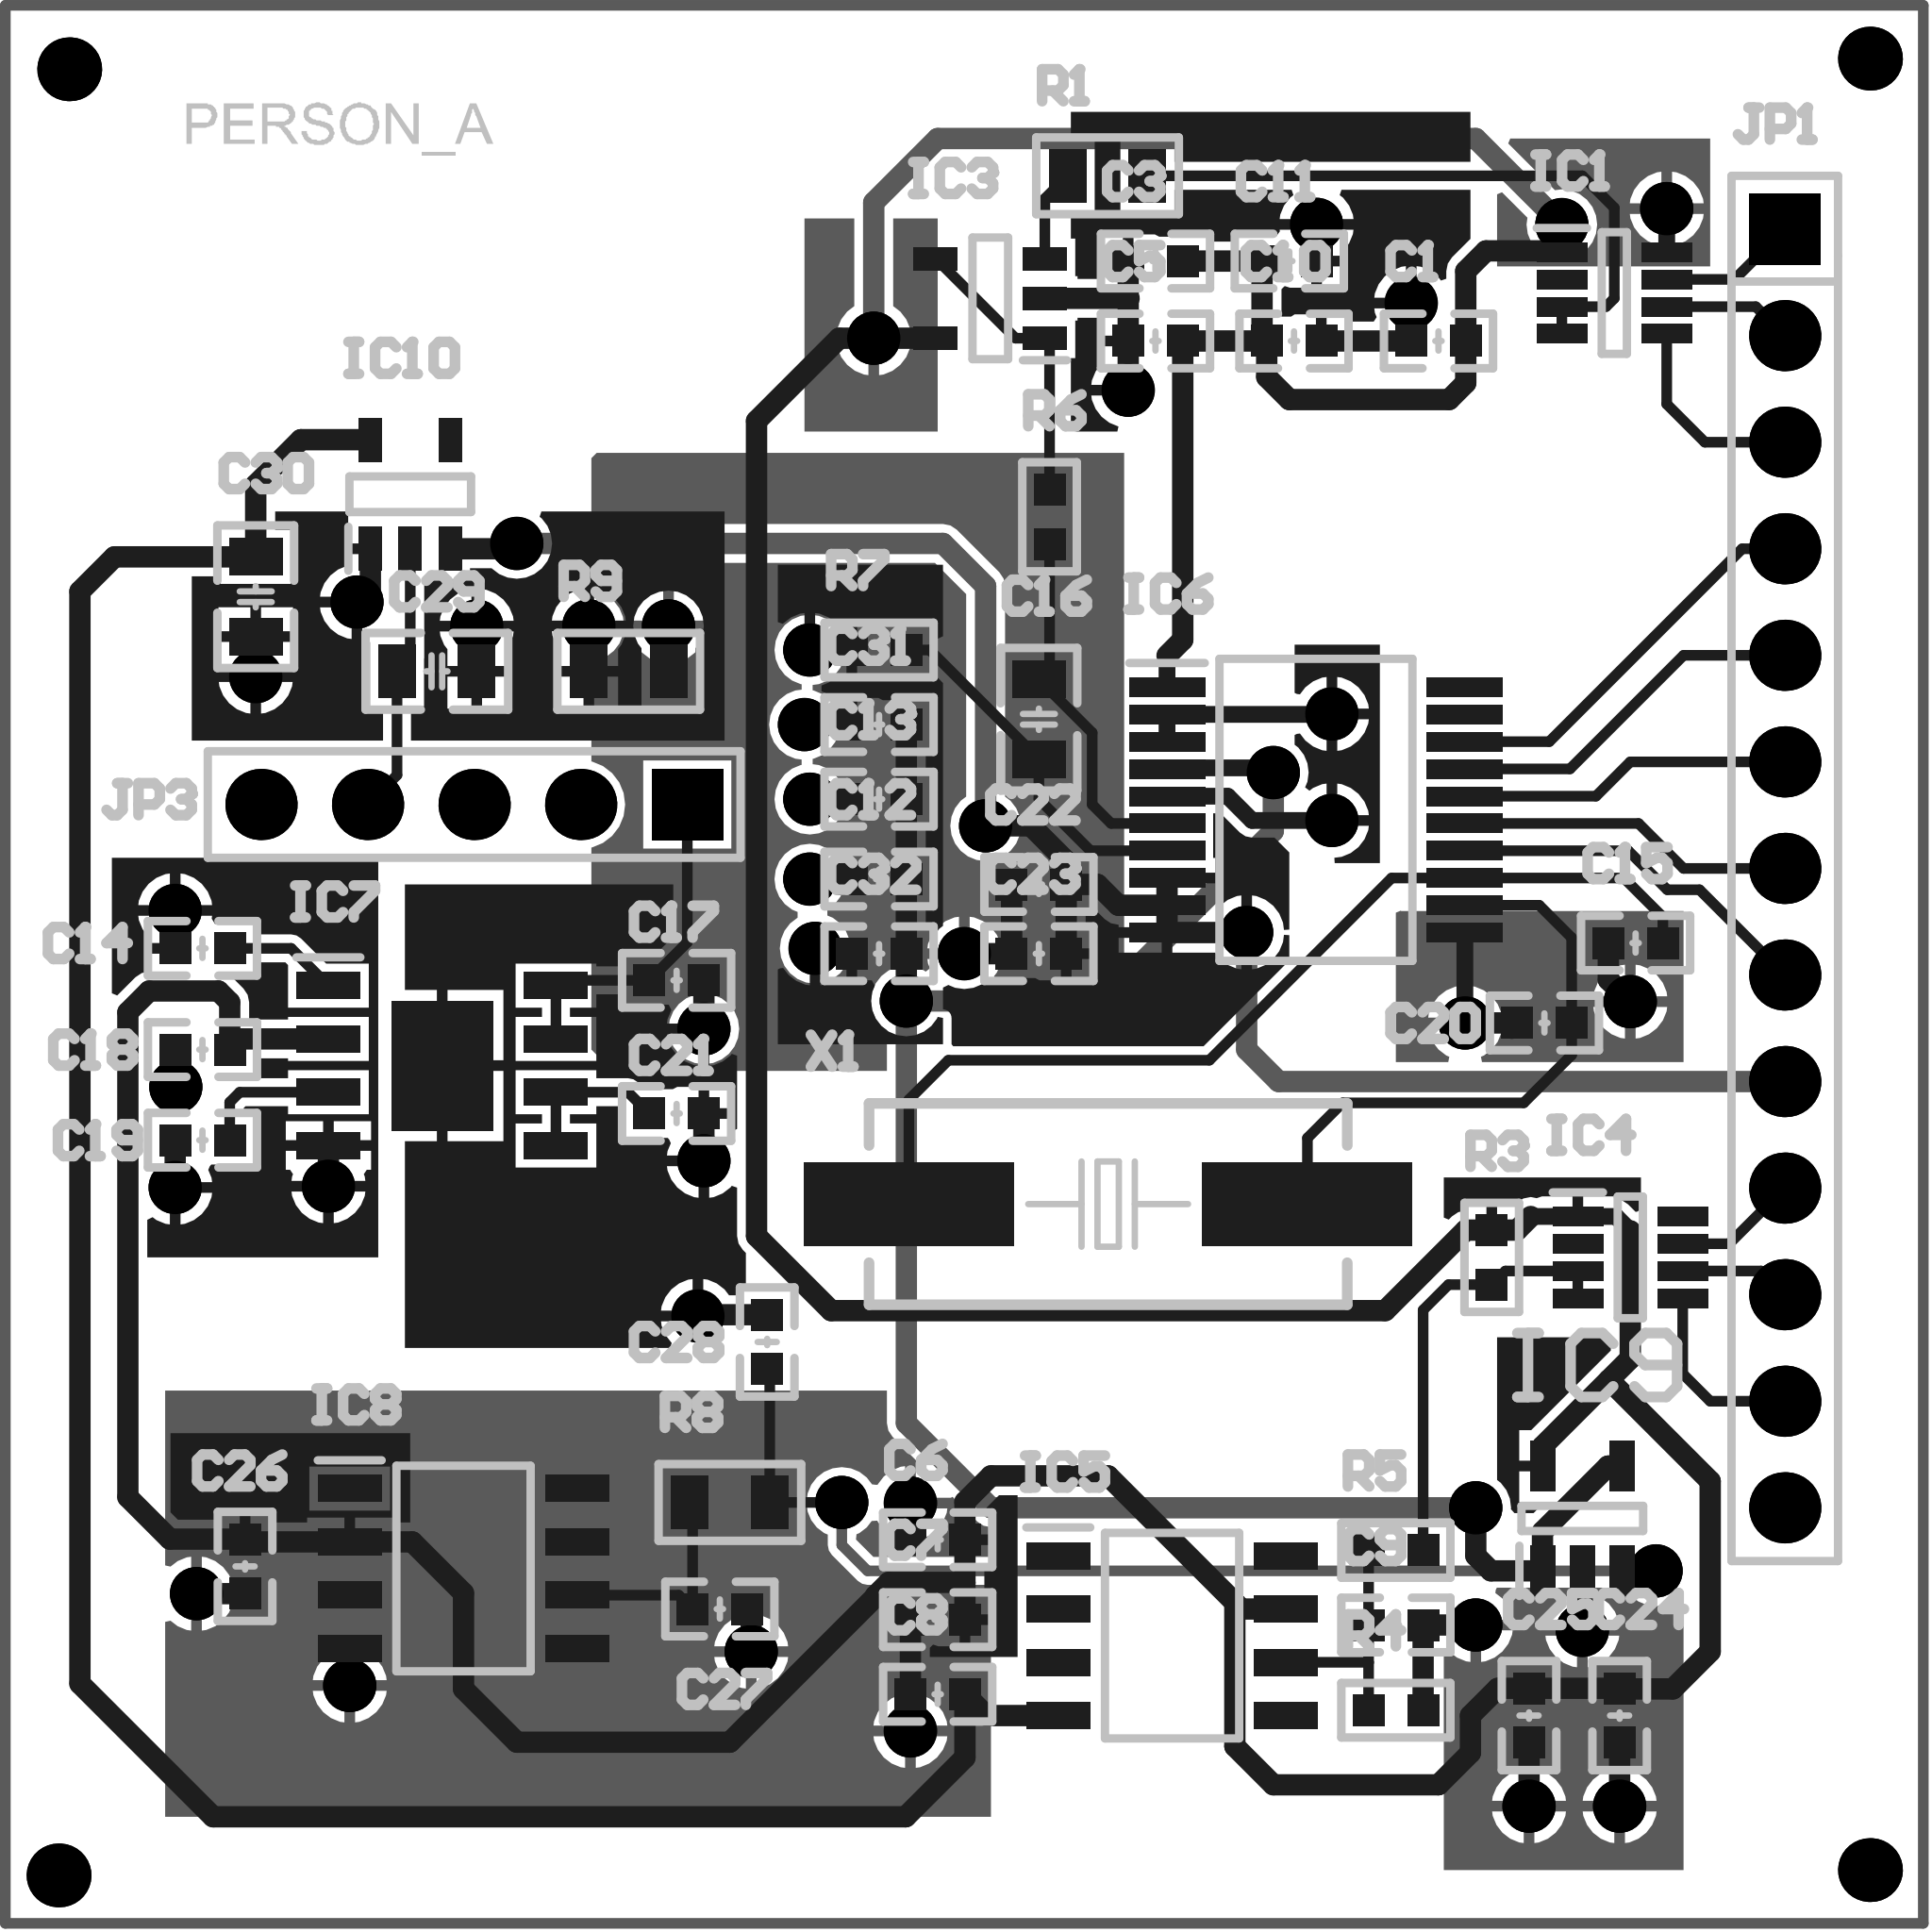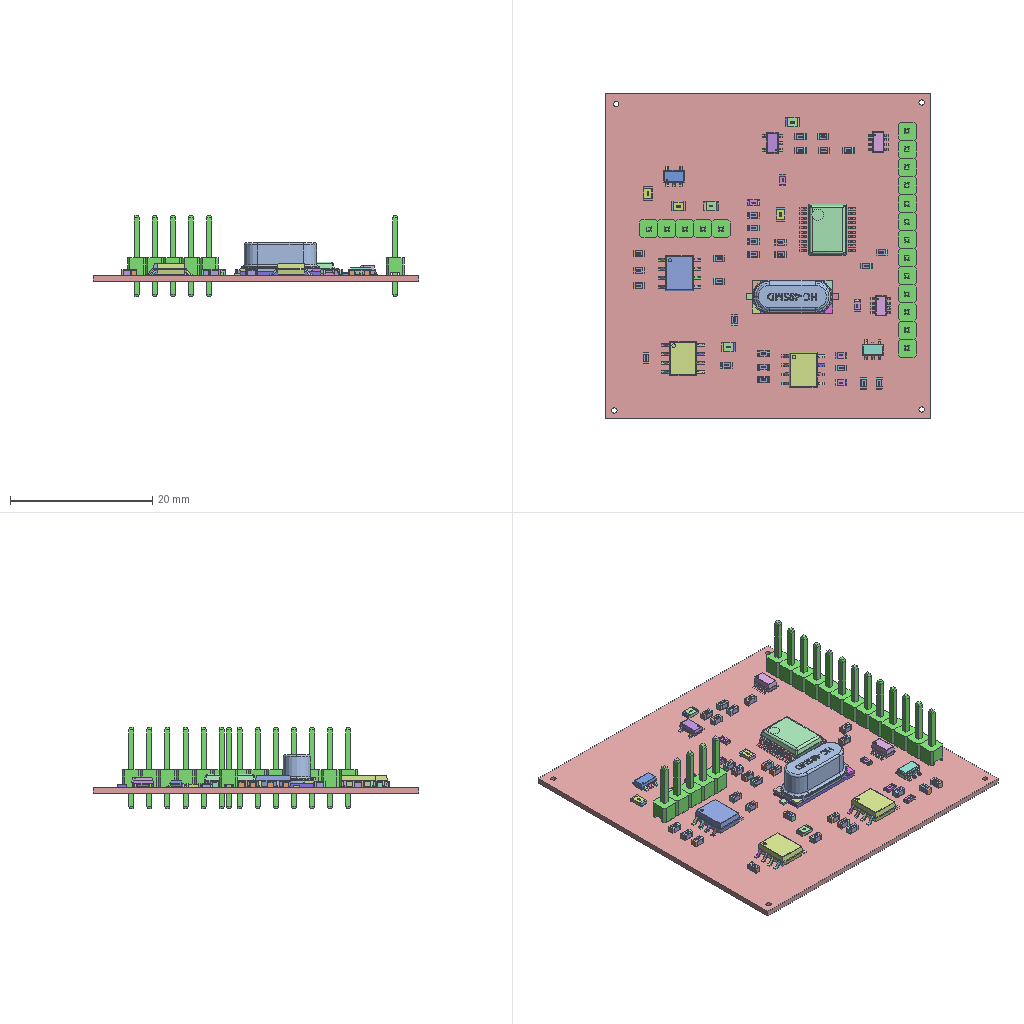Circuit board layout | Altium Designer | box 45.7 x 45.7 x 11.5 mm
Layer stack:
# Altium Designer layer stack of  (unit mm; dielectric type: 0 none, 1 core, 2 prepreg, 3 surface material)
index,name,kind,layer,copper_thickness_mm,dielectric_type,dielectric_thickness_mm,dielectric_material,dielectric_constant
0,Top Paste,other,,,,,,
1,Top Overlay,other,,,,,,
2,Top Solder,dielectric,,,3,0.0102,Solder Resist,3.5
3,Top Layer,copper,Top Layer,0.0356,,,,
4,Dielectric 1,dielectric,,,1,0.254,FR-4,4.2
5,GND,copper,GND,0.036,,,,
6,Dielectric 3,dielectric,,,2,0.127,,4.2
7,PWR,copper,PWR,0.036,,,,
8,Dielectric 2,dielectric,,,1,0.254,,4.2
9,Bottom Layer,copper,Bottom Layer,0.0356,,,,
10,Bottom Solder,dielectric,,,3,0.0102,Solder Resist,3.5
11,Bottom Overlay,other,,,,,,
12,Bottom Paste,other,,,,,,
# drill layer pairs: low layer,high layer
drill_pair,Top Layer,Bottom Layer
Part placement:
Designator,Comment,Layer,Footprint,Center-X(mm),Center-Y(mm),Rotation
IC7,ADM7150ARDZ-5.0-R7,TopLayer,SOIC127P600X175-9N,10.414,20.447,360
C1,0.1uF,TopLayer,C_0603_L,34.163,37.719,180
C6,0.1uF,TopLayer,C_0603_L,22.225,9.144,180
C7,0.1uF,TopLayer,C_0603_L,22.225,7.239,180
C8,0.1uF,TopLayer,C_0603_L,22.225,5.461,360
C9,0.1uF,TopLayer,C_0603_L,33.147,7.112,360
C12,1uF,TopLayer,C_0603_L,20.828,24.892,180
C13,100nF,TopLayer,C_0603_L,20.828,26.797,180
C14,10uF,TopLayer,C_0603_L,4.699,23.241,180
C15,20pF,TopLayer,C_0603_L,38.862,23.368,180
C16,220pF,TopLayer,C_0805_L,24.638,28.702,90
C17,10uF,TopLayer,C_0603_L,16.002,22.479,360
C18,10uF,TopLayer,C_0603_L,4.699,20.828,180
C19,1uF,TopLayer,C_0603_L,4.699,18.669,180
C20,20pF,TopLayer,C_0603_L,36.688,21.463,180
C21,1uF,TopLayer,C_0603_L,16.002,19.304,360
C22,100nF,TopLayer,C_0603_L,24.638,24.765,180
C23,1uF,TopLayer,C_0603_L,24.638,23.114,180
C24,1uF,TopLayer,C_0603_L,38.481,4.953,270
C25,100nF,TopLayer,C_0603_L,36.322,4.953,270
C26,100nF,TopLayer,C_0603_L,5.715,8.509,270
C27,100nF,TopLayer,C_0603_L,17.033,7.493,360
C28,100nF,TopLayer,C_0603_L,18.161,13.858,90
C29,2.2uF,TopLayer,C_0805_L,10.287,29.845,180
C30,2.2uF,TopLayer,C_0805_L,5.969,31.623,270
C31,10uF,TopLayer,C_0603_L,20.828,28.575,360
C32,100nF,TopLayer,C_0603_L,20.828,23.114,360
IC1,AD5660ARJZ-2500RL7,TopLayer,SOT65P280X145-8N,38.354,38.862,360
IC4,AD5660ARJZ-2500RL7,TopLayer,SOT65P280X145-8N,38.735,15.875,0
IC6,ADS1255IDBR,TopLayer,SOP65P780X200-20N,31.242,26.543,0
IC10,ADP7182AUJZ-5.0-R7,TopLayer,SOT95P280X100-5N,9.652,34.066,90
JP1,HDR-1X13,TopLayer,HDR2.54-LI-13P,42.418,25.146,270
JP3,HDR-1X5,TopLayer,HDR2.54-LI-5P,11.176,26.67,180
R3,10K,TopLayer,R_0603_L,35.433,15.875,90
R4,1K,TopLayer,R_0603_L,33.147,5.08,180
R5,10K,TopLayer,R_0603_L,33.147,8.89,360
R6,10R,TopLayer,R_0603_L,24.892,33.528,270
R7,10R,TopLayer,R_0603_L,20.828,30.353,0
R8,10K,TopLayer,R_0805_L,17.272,10.033,360
R9,0R,TopLayer,R_0805_L,14.859,29.845,360
X1,7.68MHz,TopLayer,OSC_HC-49SMD,26.289,17.145,180
IC8,ADR4525ARZ,TopLayer,SOIC127P600X175-8N,10.922,8.458,0
IC5,AD820ARZ,TopLayer,SOIC127P600X175-8N,27.813,6.858,360
C3,100nF,TopLayer,C_0603_L,27.417,39.624,180
C5,1uF,TopLayer,C_0603_L,27.417,37.719,180
C10,1uF,TopLayer,C_0603_L,30.719,37.719,360
C11,100nF,TopLayer,C_0603_L,30.607,39.624,360
IC3,OPA387DBVT,TopLayer,SOT95P280X100-5N,23.48,38.735,180
R1,50R,TopLayer,R_0805_L,26.274,41.656,180
IC9,OPA387DBVT,TopLayer,SOT95P280X145-5N,37.592,9.652,90
Pad and via stacks:
# Altium Designer via and pad stacks of  (unit mm). Each distinct definition once, with the count of objects using it.
# via: kind,start_layer,end_layer,hole_mm,diameter_mm,mode(0 simple;1 top-mid-bottom;2 full stack),diameter_per_layer,count,example_net
# pad: kind,layer,hole_mm,hole_type(0 round;1 square;2 slot),plating,top_size,top_shape(1 round;2 rect;3 octagon;9 rounded rect),mid_size,bottom_size,mode,footprint,size_per_layer,count,example
pad,Top Layer,0,0,plated,0.762x0.762,2,0.762x0.762,0.762x0.762,0,C 0603_L,,54,C32.1
pad,Top Layer,0,0,plated,1.27x0.889,2,1.27x0.889,1.27x0.889,0,C 0805_L,,6,C29.1
pad,Top Layer,0,0,unplated,1.525x0.65,2,1.525x0.65,1.525x0.65,0,SOIC127P600X175-9N,,8,IC7.1
pad,Top Layer,0,0,unplated,3.098x2.41,2,3.098x2.41,3.098x2.41,0,SOIC127P600X175-9N,,1,IC7.9
pad,Top Layer,0,0,unplated,1.525x0.65,2,1.525x0.65,1.525x0.65,0,SOIC127P600X175-8N,,16,IC5.1
pad,Top Layer,0,0,unplated,1.2x0.45,2,1.2x0.45,1.2x0.45,0,SOT65P280X145-8N,,16,IC1.1
pad,Top Layer,0,0,plated,0.762x0.762,2,0.762x0.762,0.762x0.762,0,R 0603_L,,10,R3.1
pad,Top Layer,0,0,unplated,1.8x0.45,2,1.8x0.45,1.8x0.45,0,SOP65P780X200-20N,,20,IC6.1
pad,Top Layer,0,0,plated,5x2,2,5x2,5x2,0,OSC HC-49SMD,,2,X1.1
pad,Top Layer,0,0,plated,1.27x0.889,2,1.27x0.889,1.27x0.889,0,R 0805_L,,6,R8.2
pad,Top Layer,0,0,unplated,1.05x0.55,2,1.05x0.55,1.05x0.55,0,SOT95P280X100-5N,,10,IC10.1
pad,Top Layer,0,0,unplated,1.2x0.6,2,1.2x0.6,1.2x0.6,0,SOT95P280X145-5N,,5,IC9.1
pad,Multi-Layer,0.9,0,plated,1.7x1.7,2,1.7x1.7,1.7x1.7,0,HDR2.54-LI-5P,,1,JP3.1
pad,Multi-Layer,0.9,0,plated,1.7x1.7,1,1.7x1.7,1.7x1.7,0,HDR2.54-LI-5P,,4,JP3.2
pad,Multi-Layer,0.762,0,plated,1.524x1.524,1,1.524x1.524,1.524x1.524,0,,,4,2
pad,Multi-Layer,0.9,0,plated,1.7x1.7,1,1.7x1.7,1.7x1.7,0,HDR2.54-LI-13P,,12,JP1.13
pad,Multi-Layer,0.9,0,plated,1.7x1.7,2,1.7x1.7,1.7x1.7,0,HDR2.54-LI-13P,,1,JP1.1
via,Top Layer,Bottom Layer,0.71,1.27,0,,46,DGND
Copper pours:
name,layer,net,type(0 solid;1 hatched;2 none)
D,Top Layer,D+3V3,0
G,Top Layer,AGND,0
G,Top Layer,AGND,0
G,Top Layer,A+5V,0
G,Top Layer,A+5V,0
G,Top Layer,A+5V,0
G,Top Layer,A+5V,0
G,Top Layer,AGND,0
G,Top Layer,AGND,0
G,Top Layer,AGND,0
G,Top Layer,AGND,0
D,Bottom Layer,A+5V,0
D,Bottom Layer,DGND,0
D,Bottom Layer,AGND,0
D,Bottom Layer,AGND,0
D,Bottom Layer,DGND,0
D,Bottom Layer,DGND,0
Design rules, without the lines most boards share:
# Altium Designer design rules of  (exported by Altium Designer, unit mm)
# columns: name | kind | enabled | priority | scope1 | scope2 | descriptor | typed fields (field=value)
Clearance | 0 | enabled | 1 | All | All | Clearance Constraint (Gap=0.2mm) (All),(All) | gap=0.2
PlaneConnect | 6 | enabled | 1 | All | All | Power Plane Connect Rule(Relief Connect )(Expansion=0.508mm) (Conductor Width=0.254mm) (Air Gap=0.254mm) (Entries=4) (All) | relief_conductor_width=0.254 relief_entries=4 relief_expansion=0.508
PlaneClearance | 12 | enabled | 1 | All | All | Power Plane Clearance (Clearance =0.508mm) (All) | clearance=0.508
PolygonConnect | 20 | enabled | 1 | All | All | Polygon Connect Rule(Relief Connect )(Conductor Width=0.254mm) (Relief Angle=90 Angle) (Entries=4) (Air Gap Width=0.254mm) (All),(All) | connect_style(0=relief,1=direct,2=none)=0 relief_conductor_width=0.254 relief_entries=4
PWR | 2 | enabled | 1 | InNetClass('PWR') | All | Width Constraint (Min=0.4mm) (Max=0.51mm) (Preferred=0.508mm) (InNetClass('PWR')) |
RoutingCorners | 10 | enabled | 1 | All | All | Routing Corners (Style=45-Degree) (Min Setback=2.54mm) (Max Setback=2.54mm) (All) |
RoutingVias | 11 | enabled | 1 | All | All | Routing Via (MinHoleWidth=0.711mm) (MaxHoleWidth=0.711mm) (PreferredHoleWidth=0.711mm) (MinWidth=1.27mm) (MaxWidth=1.27mm) (PreferedWidth=1.27mm) (All) | via_min_hole=0.7112 via_max_hole=0.7112 via_preferred_diameter=1.27 via_preferred_hole=0.7112
PasteMaskExpansion | 14 | enabled | 1 | All | All | Paste Mask Expansion (Expansion =0mm) (All) | expansion=0
SolderMaskExpansion | 13 | enabled | 1 | All | All | Solder Mask Expansion (Expansion =0.102mm) (All) | expansion=0.1016
ComponentClearance | 24 | enabled | 1 | All | All | Component Clearance Constraint ( Horizontal Gap = 0.254mm, Vertical Gap = 0.254mm ) (All),(All)  | gap=0.254
Height | 50 | enabled | 1 | All | All | Height Constraint (Min=0mm) (Max=25.4mm) (Prefered=12.7mm) (All) | min_height=0 max_height=25.4
HoleSize | 42 | enabled | 1 | All | All | Hole Size Constraint (Min=0.025mm) (Max=2.54mm) (All) |
DiffPairsRouting | 51 | enabled | 1 | All | All | Differential Pairs Uncoupled Length using the Gap Constraints (Min=0.254mm) (Max=0.254mm) (Prefered=0.254mm)  and Width Constraints (Min=0.381mm) (Max=0.381mm) (Prefered=0.381mm) (All) |
HoleToHoleClearance | 52 | enabled | 1 | All | All | Hole To Hole Clearance (Gap=0.508mm) (All),(All) | gap=0.508
MinimumSolderMaskSliver | 53 | enabled | 1 | All | All | Minimum Solder Mask Sliver (Gap=0mm) (All),(All) |
SilkToSolderMaskClearance | 54 | enabled | 1 | IsPad | All | Silk To Solder Mask (Clearance=0mm) (IsPad),(All) |
SilkToSilkClearance | 55 | enabled | 1 | All | All | Silk to Silk (Clearance=0mm) (All),(All) |
NetAntennae | 56 | enabled | 1 | All | All | Net Antennae (Tolerance=0mm) (All) |
Width_1 | 2 | enabled | 2 | All | All | Width Constraint (Min=0.254mm) (Max=0.51mm) (Preferred=0.254mm) (All) |
Classes set for this board:
# Altium Designer classes of  (member kind: 0 net, 1 component, 2 from-to, 3 pad, 4 layer, 5 differential pair, 6 design channel, 7 polygon, 8 structure, 9 xSignal)
# columns: class name | member kind | superclass | members
Sheet1 | 1 | no | C1; C6; C7; C8; C9; C12; C13; C14; C15; C16; C17; C18; C19; C20; C21; C22; C23; C24; C25; C26; C27; C28; C29; C30; C31; C32; IC1; IC4; IC6; IC10; JP1; JP3; R3; R4; R5; R6; R7; R8; R9; X1; IC8; IC5; C3; C5; C10; C11; IC3; IC7; IC9; R1;
PWR | 0 | no | A+5V; AGND; D-5V; DGND; REF+2V5;